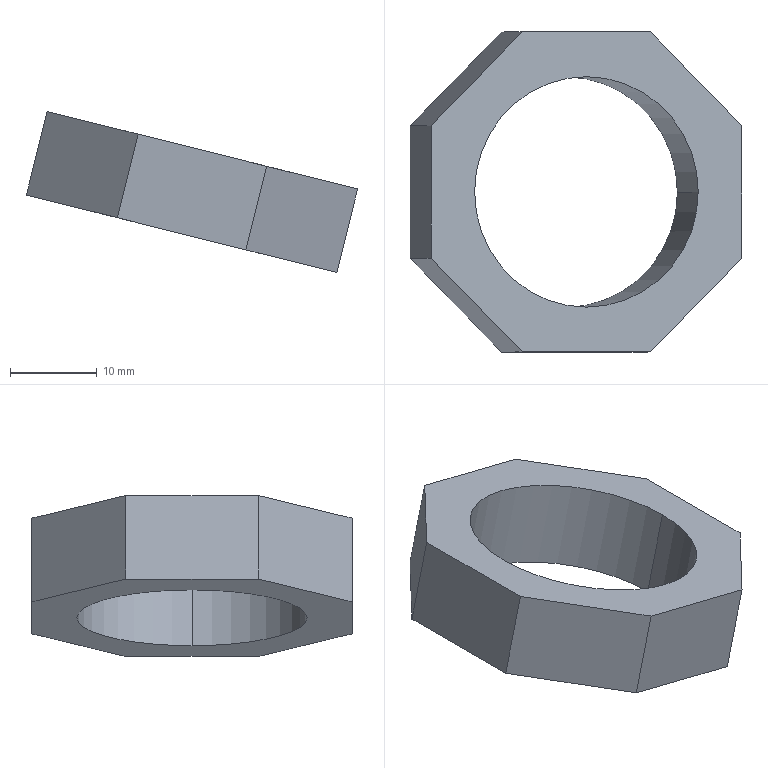Part | SolidWorks | features BaseBody 1 | 1 solid | 12 faces | box 38.102 x 36.8 x 18.507 mm | volume 5646 mm3 | plane 10 | cylinder 2 | commonest cylinder face diameters 26.5 x2
STEP:
#1=CARTESIAN_POINT('',(-436.358,-4.,313.666));
#2=VERTEX_POINT('',#1);
#3=CARTESIAN_POINT('',(-462.071,-4.,320.076));
#4=VERTEX_POINT('',#3);
#5=CARTESIAN_POINT('',(-449.215,-4.,316.871));
#6=DIRECTION('',(0.2419,0.,0.9703));
#7=DIRECTION('',(0.9703,0.,-0.2419));
#8=AXIS2_PLACEMENT_3D('',#5,#6,#7);
#9=CIRCLE('',#8,13.25);
#10=EDGE_CURVE('',#2,#4,#9,.T.);
#11=ORIENTED_EDGE('',*,*,#10,.F.);
#12=CARTESIAN_POINT('',(-433.963,-4.,323.272));
#13=VERTEX_POINT('',#12);
#14=CARTESIAN_POINT('',(-436.358,-4.,313.666));
#15=DIRECTION('',(0.2419,0.,0.9703));
#16=VECTOR('',#15,1000.);
#17=LINE('',#14,#16);
#18=EDGE_CURVE('',#2,#13,#17,.T.);
#19=ORIENTED_EDGE('',*,*,#18,.T.);
#20=CARTESIAN_POINT('',(-459.676,-4.,329.682));
#21=VERTEX_POINT('',#20);
#22=CARTESIAN_POINT('',(-446.82,-4.,326.477));
#23=DIRECTION('',(0.2419,0.,0.9703));
#24=DIRECTION('',(0.9703,0.,-0.2419));
#25=AXIS2_PLACEMENT_3D('',#22,#23,#24);
#26=CIRCLE('',#25,13.25);
#27=EDGE_CURVE('',#13,#21,#26,.T.);
#28=ORIENTED_EDGE('',*,*,#27,.T.);
#29=CARTESIAN_POINT('',(-462.071,-4.,320.076));
#30=DIRECTION('',(0.2419,0.,0.9703));
#31=VECTOR('',#30,1000.);
#32=LINE('',#29,#31);
#33=EDGE_CURVE('',#4,#21,#32,.T.);
#34=ORIENTED_EDGE('',*,*,#33,.F.);
#35=EDGE_LOOP('',(#11,#19,#28,#34));
#36=FACE_OUTER_BOUND('',#35,.T.);
#37=CARTESIAN_POINT('',(-449.215,-4.,316.871));
#38=DIRECTION('',(0.2419,0.,0.9703));
#39=DIRECTION('',(-0.9703,0.,0.2419));
#40=AXIS2_PLACEMENT_3D('',#37,#38,#39);
#41=CYLINDRICAL_SURFACE('',#40,13.25);
#42=ADVANCED_FACE('',(#36),#41,.F.);
#43=CARTESIAN_POINT('',(-446.82,-4.,326.477));
#44=DIRECTION('',(0.2419,0.,0.9703));
#45=DIRECTION('',(0.9703,0.,-0.2419));
#46=AXIS2_PLACEMENT_3D('',#43,#44,#45);
#47=CIRCLE('',#46,13.25);
#48=EDGE_CURVE('',#21,#13,#47,.T.);
#49=ORIENTED_EDGE('',*,*,#48,.F.);
#50=ORIENTED_EDGE('',*,*,#27,.F.);
#51=EDGE_LOOP('',(#49,#50));
#52=FACE_BOUND('',#51,.T.);
#53=CARTESIAN_POINT('',(-464.674,3.622,330.927));
#54=VERTEX_POINT('',#53);
#55=CARTESIAN_POINT('',(-464.674,-11.622,330.927));
#56=VERTEX_POINT('',#55);
#57=CARTESIAN_POINT('',(-464.674,-4.,330.927));
#58=DIRECTION('',(0.,-1.,0.));
#59=VECTOR('',#58,1000.);
#60=LINE('',#57,#59);
#61=EDGE_CURVE('',#54,#56,#60,.T.);
#62=ORIENTED_EDGE('',*,*,#61,.T.);
#63=CARTESIAN_POINT('',(-454.215,-22.4,328.32));
#64=VERTEX_POINT('',#63);
#65=CARTESIAN_POINT('',(-459.444,-17.011,329.624));
#66=DIRECTION('',(0.6861,-0.7071,-0.171));
#67=VECTOR('',#66,1000.);
#68=LINE('',#65,#67);
#69=EDGE_CURVE('',#56,#64,#68,.T.);
#70=ORIENTED_EDGE('',*,*,#69,.T.);
#71=CARTESIAN_POINT('',(-439.425,-22.4,324.633));
#72=VERTEX_POINT('',#71);
#73=CARTESIAN_POINT('',(-446.82,-22.4,326.477));
#74=DIRECTION('',(0.9703,0.,-0.2419));
#75=VECTOR('',#74,1000.);
#76=LINE('',#73,#75);
#77=EDGE_CURVE('',#64,#72,#76,.T.);
#78=ORIENTED_EDGE('',*,*,#77,.T.);
#79=CARTESIAN_POINT('',(-428.966,-11.622,322.026));
#80=VERTEX_POINT('',#79);
#81=CARTESIAN_POINT('',(-434.195,-17.011,323.33));
#82=DIRECTION('',(0.6861,0.7071,-0.171));
#83=VECTOR('',#82,1000.);
#84=LINE('',#81,#83);
#85=EDGE_CURVE('',#72,#80,#84,.T.);
#86=ORIENTED_EDGE('',*,*,#85,.T.);
#87=CARTESIAN_POINT('',(-428.966,3.622,322.026));
#88=VERTEX_POINT('',#87);
#89=CARTESIAN_POINT('',(-428.966,-4.,322.026));
#90=DIRECTION('',(0.,1.,0.));
#91=VECTOR('',#90,1000.);
#92=LINE('',#89,#91);
#93=EDGE_CURVE('',#80,#88,#92,.T.);
#94=ORIENTED_EDGE('',*,*,#93,.T.);
#95=CARTESIAN_POINT('',(-439.425,14.4,324.633));
#96=VERTEX_POINT('',#95);
#97=CARTESIAN_POINT('',(-434.195,9.011,323.33));
#98=DIRECTION('',(-0.6861,0.7071,0.171));
#99=VECTOR('',#98,1000.);
#100=LINE('',#97,#99);
#101=EDGE_CURVE('',#88,#96,#100,.T.);
#102=ORIENTED_EDGE('',*,*,#101,.T.);
#103=CARTESIAN_POINT('',(-454.215,14.4,328.32));
#104=VERTEX_POINT('',#103);
#105=CARTESIAN_POINT('',(-446.82,14.4,326.477));
#106=DIRECTION('',(-0.9703,0.,0.2419));
#107=VECTOR('',#106,1000.);
#108=LINE('',#105,#107);
#109=EDGE_CURVE('',#96,#104,#108,.T.);
#110=ORIENTED_EDGE('',*,*,#109,.T.);
#111=CARTESIAN_POINT('',(-459.444,9.011,329.624));
#112=DIRECTION('',(-0.6861,-0.7071,0.171));
#113=VECTOR('',#112,1000.);
#114=LINE('',#111,#113);
#115=EDGE_CURVE('',#104,#54,#114,.T.);
#116=ORIENTED_EDGE('',*,*,#115,.T.);
#117=EDGE_LOOP('',(#62,#70,#78,#86,#94,#102,#110,#116));
#118=FACE_OUTER_BOUND('',#117,.T.);
#119=CARTESIAN_POINT('',(-446.82,-4.,326.477));
#120=DIRECTION('',(0.2419,0.,0.9703));
#121=DIRECTION('',(0.,-1.,0.));
#122=AXIS2_PLACEMENT_3D('',#119,#120,#121);
#123=PLANE('',#122);
#124=ADVANCED_FACE('',(#52,#118),#123,.T.);
#125=CARTESIAN_POINT('',(-449.215,-4.,316.871));
#126=DIRECTION('',(0.2419,0.,0.9703));
#127=DIRECTION('',(0.9703,0.,-0.2419));
#128=AXIS2_PLACEMENT_3D('',#125,#126,#127);
#129=CIRCLE('',#128,13.25);
#130=EDGE_CURVE('',#4,#2,#129,.T.);
#131=ORIENTED_EDGE('',*,*,#130,.T.);
#132=ORIENTED_EDGE('',*,*,#10,.T.);
#133=EDGE_LOOP('',(#131,#132));
#134=FACE_BOUND('',#133,.T.);
#135=CARTESIAN_POINT('',(-467.068,3.622,321.321));
#136=VERTEX_POINT('',#135);
#137=CARTESIAN_POINT('',(-467.068,-11.622,321.321));
#138=VERTEX_POINT('',#137);
#139=CARTESIAN_POINT('',(-467.068,-4.,321.321));
#140=DIRECTION('',(0.,-1.,0.));
#141=VECTOR('',#140,1000.);
#142=LINE('',#139,#141);
#143=EDGE_CURVE('',#136,#138,#142,.T.);
#144=ORIENTED_EDGE('',*,*,#143,.F.);
#145=CARTESIAN_POINT('',(-456.61,14.4,318.714));
#146=VERTEX_POINT('',#145);
#147=CARTESIAN_POINT('',(-461.839,9.011,320.018));
#148=DIRECTION('',(-0.6861,-0.7071,0.171));
#149=VECTOR('',#148,1000.);
#150=LINE('',#147,#149);
#151=EDGE_CURVE('',#146,#136,#150,.T.);
#152=ORIENTED_EDGE('',*,*,#151,.F.);
#153=CARTESIAN_POINT('',(-441.819,14.4,315.027));
#154=VERTEX_POINT('',#153);
#155=CARTESIAN_POINT('',(-449.215,14.4,316.871));
#156=DIRECTION('',(-0.9703,0.,0.2419));
#157=VECTOR('',#156,1000.);
#158=LINE('',#155,#157);
#159=EDGE_CURVE('',#154,#146,#158,.T.);
#160=ORIENTED_EDGE('',*,*,#159,.F.);
#161=CARTESIAN_POINT('',(-431.361,3.622,312.42));
#162=VERTEX_POINT('',#161);
#163=CARTESIAN_POINT('',(-436.59,9.011,313.724));
#164=DIRECTION('',(-0.6861,0.7071,0.171));
#165=VECTOR('',#164,1000.);
#166=LINE('',#163,#165);
#167=EDGE_CURVE('',#162,#154,#166,.T.);
#168=ORIENTED_EDGE('',*,*,#167,.F.);
#169=CARTESIAN_POINT('',(-431.361,-11.622,312.42));
#170=VERTEX_POINT('',#169);
#171=CARTESIAN_POINT('',(-431.361,-4.,312.42));
#172=DIRECTION('',(0.,1.,0.));
#173=VECTOR('',#172,1000.);
#174=LINE('',#171,#173);
#175=EDGE_CURVE('',#170,#162,#174,.T.);
#176=ORIENTED_EDGE('',*,*,#175,.F.);
#177=CARTESIAN_POINT('',(-441.819,-22.4,315.027));
#178=VERTEX_POINT('',#177);
#179=CARTESIAN_POINT('',(-436.59,-17.011,313.724));
#180=DIRECTION('',(0.6861,0.7071,-0.171));
#181=VECTOR('',#180,1000.);
#182=LINE('',#179,#181);
#183=EDGE_CURVE('',#178,#170,#182,.T.);
#184=ORIENTED_EDGE('',*,*,#183,.F.);
#185=CARTESIAN_POINT('',(-456.61,-22.4,318.714));
#186=VERTEX_POINT('',#185);
#187=CARTESIAN_POINT('',(-449.215,-22.4,316.871));
#188=DIRECTION('',(0.9703,0.,-0.2419));
#189=VECTOR('',#188,1000.);
#190=LINE('',#187,#189);
#191=EDGE_CURVE('',#186,#178,#190,.T.);
#192=ORIENTED_EDGE('',*,*,#191,.F.);
#193=CARTESIAN_POINT('',(-461.839,-17.011,320.018));
#194=DIRECTION('',(0.6861,-0.7071,-0.171));
#195=VECTOR('',#194,1000.);
#196=LINE('',#193,#195);
#197=EDGE_CURVE('',#138,#186,#196,.T.);
#198=ORIENTED_EDGE('',*,*,#197,.F.);
#199=EDGE_LOOP('',(#144,#152,#160,#168,#176,#184,#192,#198));
#200=FACE_OUTER_BOUND('',#199,.T.);
#201=CARTESIAN_POINT('',(-449.215,-4.,316.871));
#202=DIRECTION('',(0.2419,0.,0.9703));
#203=DIRECTION('',(0.,-1.,0.));
#204=AXIS2_PLACEMENT_3D('',#201,#202,#203);
#205=PLANE('',#204);
#206=ADVANCED_FACE('',(#134,#200),#205,.F.);
#207=ORIENTED_EDGE('',*,*,#115,.F.);
#208=CARTESIAN_POINT('',(-456.61,14.4,318.714));
#209=DIRECTION('',(0.2419,0.,0.9703));
#210=VECTOR('',#209,1000.);
#211=LINE('',#208,#210);
#212=EDGE_CURVE('',#146,#104,#211,.T.);
#213=ORIENTED_EDGE('',*,*,#212,.F.);
#214=ORIENTED_EDGE('',*,*,#151,.T.);
#215=CARTESIAN_POINT('',(-467.068,3.622,321.321));
#216=DIRECTION('',(0.2419,0.,0.9703));
#217=VECTOR('',#216,1000.);
#218=LINE('',#215,#217);
#219=EDGE_CURVE('',#136,#54,#218,.T.);
#220=ORIENTED_EDGE('',*,*,#219,.T.);
#221=EDGE_LOOP('',(#207,#213,#214,#220));
#222=FACE_OUTER_BOUND('',#221,.T.);
#223=CARTESIAN_POINT('',(-461.839,9.011,320.018));
#224=DIRECTION('',(-0.6861,0.7071,0.171));
#225=DIRECTION('',(0.2419,0.,0.9703));
#226=AXIS2_PLACEMENT_3D('',#223,#224,#225);
#227=PLANE('',#226);
#228=ADVANCED_FACE('',(#222),#227,.T.);
#229=ORIENTED_EDGE('',*,*,#109,.F.);
#230=CARTESIAN_POINT('',(-441.819,14.4,315.027));
#231=DIRECTION('',(0.2419,0.,0.9703));
#232=VECTOR('',#231,1000.);
#233=LINE('',#230,#232);
#234=EDGE_CURVE('',#154,#96,#233,.T.);
#235=ORIENTED_EDGE('',*,*,#234,.F.);
#236=ORIENTED_EDGE('',*,*,#159,.T.);
#237=ORIENTED_EDGE('',*,*,#212,.T.);
#238=EDGE_LOOP('',(#229,#235,#236,#237));
#239=FACE_OUTER_BOUND('',#238,.T.);
#240=CARTESIAN_POINT('',(-449.215,14.4,316.871));
#241=DIRECTION('',(0.,1.,0.));
#242=DIRECTION('',(1.,0.,0.));
#243=AXIS2_PLACEMENT_3D('',#240,#241,#242);
#244=PLANE('',#243);
#245=ADVANCED_FACE('',(#239),#244,.T.);
#246=ORIENTED_EDGE('',*,*,#101,.F.);
#247=CARTESIAN_POINT('',(-431.361,3.622,312.42));
#248=DIRECTION('',(0.2419,0.,0.9703));
#249=VECTOR('',#248,1000.);
#250=LINE('',#247,#249);
#251=EDGE_CURVE('',#162,#88,#250,.T.);
#252=ORIENTED_EDGE('',*,*,#251,.F.);
#253=ORIENTED_EDGE('',*,*,#167,.T.);
#254=ORIENTED_EDGE('',*,*,#234,.T.);
#255=EDGE_LOOP('',(#246,#252,#253,#254));
#256=FACE_OUTER_BOUND('',#255,.T.);
#257=CARTESIAN_POINT('',(-436.59,9.011,313.724));
#258=DIRECTION('',(0.6861,0.7071,-0.171));
#259=DIRECTION('',(-0.2419,0.,-0.9703));
#260=AXIS2_PLACEMENT_3D('',#257,#258,#259);
#261=PLANE('',#260);
#262=ADVANCED_FACE('',(#256),#261,.T.);
#263=ORIENTED_EDGE('',*,*,#93,.F.);
#264=CARTESIAN_POINT('',(-431.361,-11.622,312.42));
#265=DIRECTION('',(0.2419,0.,0.9703));
#266=VECTOR('',#265,1000.);
#267=LINE('',#264,#266);
#268=EDGE_CURVE('',#170,#80,#267,.T.);
#269=ORIENTED_EDGE('',*,*,#268,.F.);
#270=ORIENTED_EDGE('',*,*,#175,.T.);
#271=ORIENTED_EDGE('',*,*,#251,.T.);
#272=EDGE_LOOP('',(#263,#269,#270,#271));
#273=FACE_OUTER_BOUND('',#272,.T.);
#274=CARTESIAN_POINT('',(-431.361,-4.,312.42));
#275=DIRECTION('',(0.9703,0.,-0.2419));
#276=DIRECTION('',(0.,-1.,0.));
#277=AXIS2_PLACEMENT_3D('',#274,#275,#276);
#278=PLANE('',#277);
#279=ADVANCED_FACE('',(#273),#278,.T.);
#280=ORIENTED_EDGE('',*,*,#85,.F.);
#281=CARTESIAN_POINT('',(-441.819,-22.4,315.027));
#282=DIRECTION('',(0.2419,0.,0.9703));
#283=VECTOR('',#282,1000.);
#284=LINE('',#281,#283);
#285=EDGE_CURVE('',#178,#72,#284,.T.);
#286=ORIENTED_EDGE('',*,*,#285,.F.);
#287=ORIENTED_EDGE('',*,*,#183,.T.);
#288=ORIENTED_EDGE('',*,*,#268,.T.);
#289=EDGE_LOOP('',(#280,#286,#287,#288));
#290=FACE_OUTER_BOUND('',#289,.T.);
#291=CARTESIAN_POINT('',(-436.59,-17.011,313.724));
#292=DIRECTION('',(0.6861,-0.7071,-0.171));
#293=DIRECTION('',(0.,0.2351,-0.972));
#294=AXIS2_PLACEMENT_3D('',#291,#292,#293);
#295=PLANE('',#294);
#296=ADVANCED_FACE('',(#290),#295,.T.);
#297=ORIENTED_EDGE('',*,*,#77,.F.);
#298=CARTESIAN_POINT('',(-456.61,-22.4,318.714));
#299=DIRECTION('',(0.2419,0.,0.9703));
#300=VECTOR('',#299,1000.);
#301=LINE('',#298,#300);
#302=EDGE_CURVE('',#186,#64,#301,.T.);
#303=ORIENTED_EDGE('',*,*,#302,.F.);
#304=ORIENTED_EDGE('',*,*,#191,.T.);
#305=ORIENTED_EDGE('',*,*,#285,.T.);
#306=EDGE_LOOP('',(#297,#303,#304,#305));
#307=FACE_OUTER_BOUND('',#306,.T.);
#308=CARTESIAN_POINT('',(-449.215,-22.4,316.871));
#309=DIRECTION('',(0.,-1.,0.));
#310=DIRECTION('',(-1.,0.,0.));
#311=AXIS2_PLACEMENT_3D('',#308,#309,#310);
#312=PLANE('',#311);
#313=ADVANCED_FACE('',(#307),#312,.T.);
#314=ORIENTED_EDGE('',*,*,#69,.F.);
#315=CARTESIAN_POINT('',(-467.068,-11.622,321.321));
#316=DIRECTION('',(0.2419,0.,0.9703));
#317=VECTOR('',#316,1000.);
#318=LINE('',#315,#317);
#319=EDGE_CURVE('',#138,#56,#318,.T.);
#320=ORIENTED_EDGE('',*,*,#319,.F.);
#321=ORIENTED_EDGE('',*,*,#197,.T.);
#322=ORIENTED_EDGE('',*,*,#302,.T.);
#323=EDGE_LOOP('',(#314,#320,#321,#322));
#324=FACE_OUTER_BOUND('',#323,.T.);
#325=CARTESIAN_POINT('',(-461.839,-17.011,320.018));
#326=DIRECTION('',(-0.6861,-0.7071,0.171));
#327=DIRECTION('',(-0.7177,0.6964,0.));
#328=AXIS2_PLACEMENT_3D('',#325,#326,#327);
#329=PLANE('',#328);
#330=ADVANCED_FACE('',(#324),#329,.T.);
#331=ORIENTED_EDGE('',*,*,#61,.F.);
#332=ORIENTED_EDGE('',*,*,#219,.F.);
#333=ORIENTED_EDGE('',*,*,#143,.T.);
#334=ORIENTED_EDGE('',*,*,#319,.T.);
#335=EDGE_LOOP('',(#331,#332,#333,#334));
#336=FACE_OUTER_BOUND('',#335,.T.);
#337=CARTESIAN_POINT('',(-467.068,-4.,321.321));
#338=DIRECTION('',(-0.9703,0.,0.2419));
#339=DIRECTION('',(0.,1.,0.));
#340=AXIS2_PLACEMENT_3D('',#337,#338,#339);
#341=PLANE('',#340);
#342=ADVANCED_FACE('',(#336),#341,.T.);
#343=ORIENTED_EDGE('',*,*,#18,.F.);
#344=ORIENTED_EDGE('',*,*,#130,.F.);
#345=ORIENTED_EDGE('',*,*,#33,.T.);
#346=ORIENTED_EDGE('',*,*,#48,.T.);
#347=EDGE_LOOP('',(#343,#344,#345,#346));
#348=FACE_OUTER_BOUND('',#347,.T.);
#349=CARTESIAN_POINT('',(-449.215,-4.,316.871));
#350=DIRECTION('',(0.2419,0.,0.9703));
#351=DIRECTION('',(-0.9703,0.,0.2419));
#352=AXIS2_PLACEMENT_3D('',#349,#350,#351);
#353=CYLINDRICAL_SURFACE('',#352,13.25);
#354=ADVANCED_FACE('',(#348),#353,.F.);
#355=CLOSED_SHELL('',(#42,#124,#206,#228,#245,#262,#279,#296,#313,#330,#342,#354));
#356=MANIFOLD_SOLID_BREP('',#355);
#357=CARTESIAN_POINT('',(0.,0.,0.));
#358=DIRECTION('',(0.,0.,1.));
#359=DIRECTION('',(1.,0.,0.));
#360=AXIS2_PLACEMENT_3D('',#357,#358,#359);
#361=(LENGTH_UNIT()NAMED_UNIT(*)SI_UNIT(.MILLI.,.METRE.));
#362=UNCERTAINTY_MEASURE_WITH_UNIT(LENGTH_MEASURE(0.00001),#361,'','');
#363=(NAMED_UNIT(*)PLANE_ANGLE_UNIT()SI_UNIT($,.RADIAN.));
#364=(NAMED_UNIT(*)SI_UNIT($,.STERADIAN.)SOLID_ANGLE_UNIT());
#365=(GEOMETRIC_REPRESENTATION_CONTEXT(3)GLOBAL_UNCERTAINTY_ASSIGNED_CONTEXT((#362))GLOBAL_UNIT_ASSIGNED_CONTEXT((#361,#363,#364))REPRESENTATION_CONTEXT('',''));
#366=ADVANCED_BREP_SHAPE_REPRESENTATION('',(#356,#360),#365);